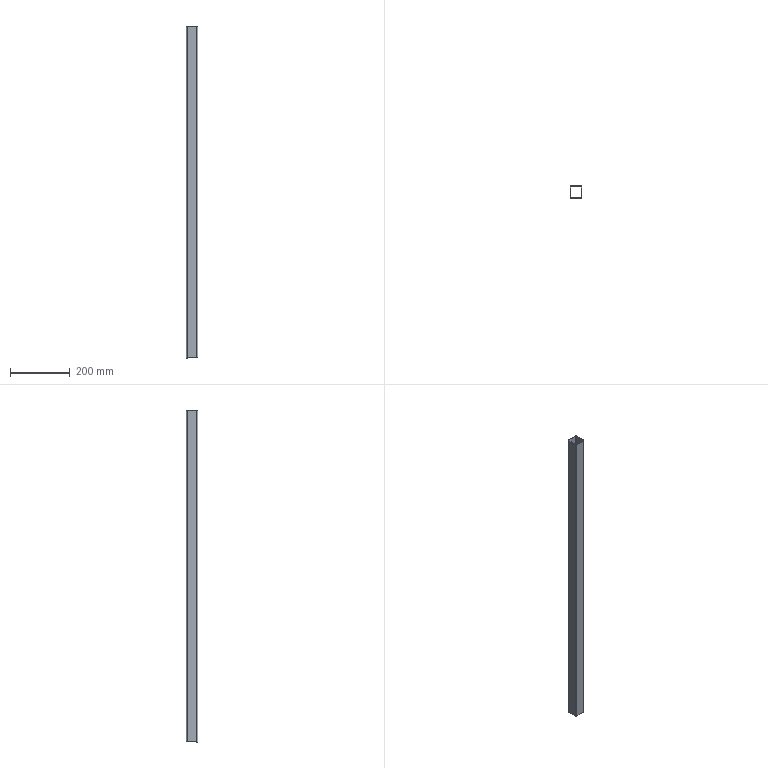Part | SolidWorks | features Fillet 2, Extrusion 1 | 1 solid | 18 faces | box 40 x 40 x 1116 mm | volume 327768 mm3 | plane 10 | cylinder 8 | commonest cylinder face diameters 4 x4 8 x4
STEP:
#1=CARTESIAN_POINT('',(20.,-16.,1116.));
#2=VERTEX_POINT('',#1);
#3=CARTESIAN_POINT('',(20.,16.,1116.));
#4=VERTEX_POINT('',#3);
#5=CARTESIAN_POINT('',(20.,20.,1116.));
#6=DIRECTION('',(0.,1.,0.));
#7=VECTOR('',#6,1000.);
#8=LINE('',#5,#7);
#9=EDGE_CURVE('',#2,#4,#8,.T.);
#10=ORIENTED_EDGE('',*,*,#9,.T.);
#11=CARTESIAN_POINT('',(16.,20.,1116.));
#12=VERTEX_POINT('',#11);
#13=CARTESIAN_POINT('',(16.,16.,1116.));
#14=DIRECTION('',(0.,0.,1.));
#15=DIRECTION('',(1.,0.,0.));
#16=AXIS2_PLACEMENT_3D('',#13,#14,#15);
#17=CIRCLE('',#16,4.);
#18=EDGE_CURVE('',#4,#12,#17,.T.);
#19=ORIENTED_EDGE('',*,*,#18,.T.);
#20=CARTESIAN_POINT('',(-16.,20.,1116.));
#21=VERTEX_POINT('',#20);
#22=CARTESIAN_POINT('',(-20.,20.,1116.));
#23=DIRECTION('',(-1.,0.,0.));
#24=VECTOR('',#23,1000.);
#25=LINE('',#22,#24);
#26=EDGE_CURVE('',#12,#21,#25,.T.);
#27=ORIENTED_EDGE('',*,*,#26,.T.);
#28=CARTESIAN_POINT('',(-20.,16.,1116.));
#29=VERTEX_POINT('',#28);
#30=CARTESIAN_POINT('',(-16.,16.,1116.));
#31=DIRECTION('',(0.,0.,1.));
#32=DIRECTION('',(1.,0.,0.));
#33=AXIS2_PLACEMENT_3D('',#30,#31,#32);
#34=CIRCLE('',#33,4.);
#35=EDGE_CURVE('',#21,#29,#34,.T.);
#36=ORIENTED_EDGE('',*,*,#35,.T.);
#37=CARTESIAN_POINT('',(-20.,-16.,1116.));
#38=VERTEX_POINT('',#37);
#39=CARTESIAN_POINT('',(-20.,20.,1116.));
#40=DIRECTION('',(0.,-1.,0.));
#41=VECTOR('',#40,1000.);
#42=LINE('',#39,#41);
#43=EDGE_CURVE('',#29,#38,#42,.T.);
#44=ORIENTED_EDGE('',*,*,#43,.T.);
#45=CARTESIAN_POINT('',(-16.,-20.,1116.));
#46=VERTEX_POINT('',#45);
#47=CARTESIAN_POINT('',(-16.,-16.,1116.));
#48=DIRECTION('',(0.,0.,1.));
#49=DIRECTION('',(1.,0.,0.));
#50=AXIS2_PLACEMENT_3D('',#47,#48,#49);
#51=CIRCLE('',#50,4.);
#52=EDGE_CURVE('',#38,#46,#51,.T.);
#53=ORIENTED_EDGE('',*,*,#52,.T.);
#54=CARTESIAN_POINT('',(16.,-20.,1116.));
#55=VERTEX_POINT('',#54);
#56=CARTESIAN_POINT('',(-20.,-20.,1116.));
#57=DIRECTION('',(1.,0.,0.));
#58=VECTOR('',#57,1000.);
#59=LINE('',#56,#58);
#60=EDGE_CURVE('',#46,#55,#59,.T.);
#61=ORIENTED_EDGE('',*,*,#60,.T.);
#62=CARTESIAN_POINT('',(16.,-16.,1116.));
#63=DIRECTION('',(0.,0.,1.));
#64=DIRECTION('',(1.,0.,0.));
#65=AXIS2_PLACEMENT_3D('',#62,#63,#64);
#66=CIRCLE('',#65,4.);
#67=EDGE_CURVE('',#55,#2,#66,.T.);
#68=ORIENTED_EDGE('',*,*,#67,.T.);
#69=EDGE_LOOP('',(#10,#19,#27,#36,#44,#53,#61,#68));
#70=FACE_OUTER_BOUND('',#69,.T.);
#71=CARTESIAN_POINT('',(16.,18.,1116.));
#72=VERTEX_POINT('',#71);
#73=CARTESIAN_POINT('',(-16.,18.,1116.));
#74=VERTEX_POINT('',#73);
#75=CARTESIAN_POINT('',(-18.,18.,1116.));
#76=DIRECTION('',(-1.,0.,0.));
#77=VECTOR('',#76,1000.);
#78=LINE('',#75,#77);
#79=EDGE_CURVE('',#72,#74,#78,.T.);
#80=ORIENTED_EDGE('',*,*,#79,.F.);
#81=CARTESIAN_POINT('',(18.,16.,1116.));
#82=VERTEX_POINT('',#81);
#83=CARTESIAN_POINT('',(16.,16.,1116.));
#84=DIRECTION('',(0.,0.,-1.));
#85=DIRECTION('',(1.,0.,0.));
#86=AXIS2_PLACEMENT_3D('',#83,#84,#85);
#87=CIRCLE('',#86,2.);
#88=EDGE_CURVE('',#72,#82,#87,.T.);
#89=ORIENTED_EDGE('',*,*,#88,.T.);
#90=CARTESIAN_POINT('',(18.,-16.,1116.));
#91=VERTEX_POINT('',#90);
#92=CARTESIAN_POINT('',(18.,18.,1116.));
#93=DIRECTION('',(0.,1.,0.));
#94=VECTOR('',#93,1000.);
#95=LINE('',#92,#94);
#96=EDGE_CURVE('',#91,#82,#95,.T.);
#97=ORIENTED_EDGE('',*,*,#96,.F.);
#98=CARTESIAN_POINT('',(16.,-18.,1116.));
#99=VERTEX_POINT('',#98);
#100=CARTESIAN_POINT('',(16.,-16.,1116.));
#101=DIRECTION('',(0.,0.,-1.));
#102=DIRECTION('',(1.,0.,0.));
#103=AXIS2_PLACEMENT_3D('',#100,#101,#102);
#104=CIRCLE('',#103,2.);
#105=EDGE_CURVE('',#91,#99,#104,.T.);
#106=ORIENTED_EDGE('',*,*,#105,.T.);
#107=CARTESIAN_POINT('',(-16.,-18.,1116.));
#108=VERTEX_POINT('',#107);
#109=CARTESIAN_POINT('',(-18.,-18.,1116.));
#110=DIRECTION('',(1.,0.,0.));
#111=VECTOR('',#110,1000.);
#112=LINE('',#109,#111);
#113=EDGE_CURVE('',#108,#99,#112,.T.);
#114=ORIENTED_EDGE('',*,*,#113,.F.);
#115=CARTESIAN_POINT('',(-18.,-16.,1116.));
#116=VERTEX_POINT('',#115);
#117=CARTESIAN_POINT('',(-16.,-16.,1116.));
#118=DIRECTION('',(0.,0.,-1.));
#119=DIRECTION('',(1.,0.,0.));
#120=AXIS2_PLACEMENT_3D('',#117,#118,#119);
#121=CIRCLE('',#120,2.);
#122=EDGE_CURVE('',#108,#116,#121,.T.);
#123=ORIENTED_EDGE('',*,*,#122,.T.);
#124=CARTESIAN_POINT('',(-18.,16.,1116.));
#125=VERTEX_POINT('',#124);
#126=CARTESIAN_POINT('',(-18.,18.,1116.));
#127=DIRECTION('',(0.,-1.,0.));
#128=VECTOR('',#127,1000.);
#129=LINE('',#126,#128);
#130=EDGE_CURVE('',#125,#116,#129,.T.);
#131=ORIENTED_EDGE('',*,*,#130,.F.);
#132=CARTESIAN_POINT('',(-16.,16.,1116.));
#133=DIRECTION('',(0.,0.,-1.));
#134=DIRECTION('',(1.,0.,0.));
#135=AXIS2_PLACEMENT_3D('',#132,#133,#134);
#136=CIRCLE('',#135,2.);
#137=EDGE_CURVE('',#125,#74,#136,.T.);
#138=ORIENTED_EDGE('',*,*,#137,.T.);
#139=EDGE_LOOP('',(#80,#89,#97,#106,#114,#123,#131,#138));
#140=FACE_BOUND('',#139,.T.);
#141=CARTESIAN_POINT('',(0.,0.,1116.));
#142=DIRECTION('',(0.,0.,1.));
#143=DIRECTION('',(1.,0.,0.));
#144=AXIS2_PLACEMENT_3D('',#141,#142,#143);
#145=PLANE('',#144);
#146=ADVANCED_FACE('',(#70,#140),#145,.T.);
#147=CARTESIAN_POINT('',(16.,20.,0.));
#148=VERTEX_POINT('',#147);
#149=CARTESIAN_POINT('',(-16.,20.,0.));
#150=VERTEX_POINT('',#149);
#151=CARTESIAN_POINT('',(-20.,20.,0.));
#152=DIRECTION('',(-1.,0.,0.));
#153=VECTOR('',#152,1000.);
#154=LINE('',#151,#153);
#155=EDGE_CURVE('',#148,#150,#154,.T.);
#156=ORIENTED_EDGE('',*,*,#155,.F.);
#157=CARTESIAN_POINT('',(20.,16.,0.));
#158=VERTEX_POINT('',#157);
#159=CARTESIAN_POINT('',(16.,16.,0.));
#160=DIRECTION('',(0.,0.,-1.));
#161=DIRECTION('',(1.,0.,0.));
#162=AXIS2_PLACEMENT_3D('',#159,#160,#161);
#163=CIRCLE('',#162,4.);
#164=EDGE_CURVE('',#148,#158,#163,.T.);
#165=ORIENTED_EDGE('',*,*,#164,.T.);
#166=CARTESIAN_POINT('',(20.,-16.,0.));
#167=VERTEX_POINT('',#166);
#168=CARTESIAN_POINT('',(20.,20.,0.));
#169=DIRECTION('',(0.,1.,0.));
#170=VECTOR('',#169,1000.);
#171=LINE('',#168,#170);
#172=EDGE_CURVE('',#167,#158,#171,.T.);
#173=ORIENTED_EDGE('',*,*,#172,.F.);
#174=CARTESIAN_POINT('',(16.,-20.,0.));
#175=VERTEX_POINT('',#174);
#176=CARTESIAN_POINT('',(16.,-16.,0.));
#177=DIRECTION('',(0.,0.,-1.));
#178=DIRECTION('',(1.,0.,0.));
#179=AXIS2_PLACEMENT_3D('',#176,#177,#178);
#180=CIRCLE('',#179,4.);
#181=EDGE_CURVE('',#167,#175,#180,.T.);
#182=ORIENTED_EDGE('',*,*,#181,.T.);
#183=CARTESIAN_POINT('',(-16.,-20.,0.));
#184=VERTEX_POINT('',#183);
#185=CARTESIAN_POINT('',(-20.,-20.,0.));
#186=DIRECTION('',(1.,0.,0.));
#187=VECTOR('',#186,1000.);
#188=LINE('',#185,#187);
#189=EDGE_CURVE('',#184,#175,#188,.T.);
#190=ORIENTED_EDGE('',*,*,#189,.F.);
#191=CARTESIAN_POINT('',(-20.,-16.,0.));
#192=VERTEX_POINT('',#191);
#193=CARTESIAN_POINT('',(-16.,-16.,0.));
#194=DIRECTION('',(0.,0.,-1.));
#195=DIRECTION('',(1.,0.,0.));
#196=AXIS2_PLACEMENT_3D('',#193,#194,#195);
#197=CIRCLE('',#196,4.);
#198=EDGE_CURVE('',#184,#192,#197,.T.);
#199=ORIENTED_EDGE('',*,*,#198,.T.);
#200=CARTESIAN_POINT('',(-20.,16.,0.));
#201=VERTEX_POINT('',#200);
#202=CARTESIAN_POINT('',(-20.,20.,0.));
#203=DIRECTION('',(0.,-1.,0.));
#204=VECTOR('',#203,1000.);
#205=LINE('',#202,#204);
#206=EDGE_CURVE('',#201,#192,#205,.T.);
#207=ORIENTED_EDGE('',*,*,#206,.F.);
#208=CARTESIAN_POINT('',(-16.,16.,0.));
#209=DIRECTION('',(0.,0.,-1.));
#210=DIRECTION('',(1.,0.,0.));
#211=AXIS2_PLACEMENT_3D('',#208,#209,#210);
#212=CIRCLE('',#211,4.);
#213=EDGE_CURVE('',#201,#150,#212,.T.);
#214=ORIENTED_EDGE('',*,*,#213,.T.);
#215=EDGE_LOOP('',(#156,#165,#173,#182,#190,#199,#207,#214));
#216=FACE_OUTER_BOUND('',#215,.T.);
#217=CARTESIAN_POINT('',(-16.,-18.,0.));
#218=VERTEX_POINT('',#217);
#219=CARTESIAN_POINT('',(16.,-18.,0.));
#220=VERTEX_POINT('',#219);
#221=CARTESIAN_POINT('',(-18.,-18.,0.));
#222=DIRECTION('',(1.,0.,0.));
#223=VECTOR('',#222,1000.);
#224=LINE('',#221,#223);
#225=EDGE_CURVE('',#218,#220,#224,.T.);
#226=ORIENTED_EDGE('',*,*,#225,.T.);
#227=CARTESIAN_POINT('',(18.,-16.,0.));
#228=VERTEX_POINT('',#227);
#229=CARTESIAN_POINT('',(16.,-16.,0.));
#230=DIRECTION('',(0.,0.,1.));
#231=DIRECTION('',(1.,0.,0.));
#232=AXIS2_PLACEMENT_3D('',#229,#230,#231);
#233=CIRCLE('',#232,2.);
#234=EDGE_CURVE('',#220,#228,#233,.T.);
#235=ORIENTED_EDGE('',*,*,#234,.T.);
#236=CARTESIAN_POINT('',(18.,16.,0.));
#237=VERTEX_POINT('',#236);
#238=CARTESIAN_POINT('',(18.,18.,0.));
#239=DIRECTION('',(0.,1.,0.));
#240=VECTOR('',#239,1000.);
#241=LINE('',#238,#240);
#242=EDGE_CURVE('',#228,#237,#241,.T.);
#243=ORIENTED_EDGE('',*,*,#242,.T.);
#244=CARTESIAN_POINT('',(16.,18.,0.));
#245=VERTEX_POINT('',#244);
#246=CARTESIAN_POINT('',(16.,16.,0.));
#247=DIRECTION('',(0.,0.,1.));
#248=DIRECTION('',(1.,0.,0.));
#249=AXIS2_PLACEMENT_3D('',#246,#247,#248);
#250=CIRCLE('',#249,2.);
#251=EDGE_CURVE('',#237,#245,#250,.T.);
#252=ORIENTED_EDGE('',*,*,#251,.T.);
#253=CARTESIAN_POINT('',(-16.,18.,0.));
#254=VERTEX_POINT('',#253);
#255=CARTESIAN_POINT('',(-18.,18.,0.));
#256=DIRECTION('',(-1.,0.,0.));
#257=VECTOR('',#256,1000.);
#258=LINE('',#255,#257);
#259=EDGE_CURVE('',#245,#254,#258,.T.);
#260=ORIENTED_EDGE('',*,*,#259,.T.);
#261=CARTESIAN_POINT('',(-18.,16.,0.));
#262=VERTEX_POINT('',#261);
#263=CARTESIAN_POINT('',(-16.,16.,0.));
#264=DIRECTION('',(0.,0.,1.));
#265=DIRECTION('',(1.,0.,0.));
#266=AXIS2_PLACEMENT_3D('',#263,#264,#265);
#267=CIRCLE('',#266,2.);
#268=EDGE_CURVE('',#254,#262,#267,.T.);
#269=ORIENTED_EDGE('',*,*,#268,.T.);
#270=CARTESIAN_POINT('',(-18.,-16.,0.));
#271=VERTEX_POINT('',#270);
#272=CARTESIAN_POINT('',(-18.,18.,0.));
#273=DIRECTION('',(0.,-1.,0.));
#274=VECTOR('',#273,1000.);
#275=LINE('',#272,#274);
#276=EDGE_CURVE('',#262,#271,#275,.T.);
#277=ORIENTED_EDGE('',*,*,#276,.T.);
#278=CARTESIAN_POINT('',(-16.,-16.,0.));
#279=DIRECTION('',(0.,0.,1.));
#280=DIRECTION('',(1.,0.,0.));
#281=AXIS2_PLACEMENT_3D('',#278,#279,#280);
#282=CIRCLE('',#281,2.);
#283=EDGE_CURVE('',#271,#218,#282,.T.);
#284=ORIENTED_EDGE('',*,*,#283,.T.);
#285=EDGE_LOOP('',(#226,#235,#243,#252,#260,#269,#277,#284));
#286=FACE_BOUND('',#285,.T.);
#287=CARTESIAN_POINT('',(0.,0.,0.));
#288=DIRECTION('',(0.,0.,1.));
#289=DIRECTION('',(1.,0.,0.));
#290=AXIS2_PLACEMENT_3D('',#287,#288,#289);
#291=PLANE('',#290);
#292=ADVANCED_FACE('',(#216,#286),#291,.F.);
#293=ORIENTED_EDGE('',*,*,#172,.T.);
#294=CARTESIAN_POINT('',(20.,16.,1116.));
#295=DIRECTION('',(0.,0.,1.));
#296=VECTOR('',#295,1000.);
#297=LINE('',#294,#296);
#298=EDGE_CURVE('',#158,#4,#297,.T.);
#299=ORIENTED_EDGE('',*,*,#298,.T.);
#300=ORIENTED_EDGE('',*,*,#9,.F.);
#301=CARTESIAN_POINT('',(20.,-16.,1116.));
#302=DIRECTION('',(0.,0.,-1.));
#303=VECTOR('',#302,1000.);
#304=LINE('',#301,#303);
#305=EDGE_CURVE('',#2,#167,#304,.T.);
#306=ORIENTED_EDGE('',*,*,#305,.T.);
#307=EDGE_LOOP('',(#293,#299,#300,#306));
#308=FACE_OUTER_BOUND('',#307,.T.);
#309=CARTESIAN_POINT('',(20.,20.,1116.));
#310=DIRECTION('',(-1.,0.,0.));
#311=DIRECTION('',(0.,0.,1.));
#312=AXIS2_PLACEMENT_3D('',#309,#310,#311);
#313=PLANE('',#312);
#314=ADVANCED_FACE('',(#308),#313,.F.);
#315=ORIENTED_EDGE('',*,*,#26,.F.);
#316=CARTESIAN_POINT('',(16.,20.,1116.));
#317=DIRECTION('',(0.,0.,-1.));
#318=VECTOR('',#317,1000.);
#319=LINE('',#316,#318);
#320=EDGE_CURVE('',#12,#148,#319,.T.);
#321=ORIENTED_EDGE('',*,*,#320,.T.);
#322=ORIENTED_EDGE('',*,*,#155,.T.);
#323=CARTESIAN_POINT('',(-16.,20.,1116.));
#324=DIRECTION('',(0.,0.,1.));
#325=VECTOR('',#324,1000.);
#326=LINE('',#323,#325);
#327=EDGE_CURVE('',#150,#21,#326,.T.);
#328=ORIENTED_EDGE('',*,*,#327,.T.);
#329=EDGE_LOOP('',(#315,#321,#322,#328));
#330=FACE_OUTER_BOUND('',#329,.T.);
#331=CARTESIAN_POINT('',(-20.,20.,1116.));
#332=DIRECTION('',(0.,-1.,0.));
#333=DIRECTION('',(0.,0.,-1.));
#334=AXIS2_PLACEMENT_3D('',#331,#332,#333);
#335=PLANE('',#334);
#336=ADVANCED_FACE('',(#330),#335,.F.);
#337=ORIENTED_EDGE('',*,*,#43,.F.);
#338=CARTESIAN_POINT('',(-20.,16.,1116.));
#339=DIRECTION('',(0.,0.,-1.));
#340=VECTOR('',#339,1000.);
#341=LINE('',#338,#340);
#342=EDGE_CURVE('',#29,#201,#341,.T.);
#343=ORIENTED_EDGE('',*,*,#342,.T.);
#344=ORIENTED_EDGE('',*,*,#206,.T.);
#345=CARTESIAN_POINT('',(-20.,-16.,1116.));
#346=DIRECTION('',(0.,0.,1.));
#347=VECTOR('',#346,1000.);
#348=LINE('',#345,#347);
#349=EDGE_CURVE('',#192,#38,#348,.T.);
#350=ORIENTED_EDGE('',*,*,#349,.T.);
#351=EDGE_LOOP('',(#337,#343,#344,#350));
#352=FACE_OUTER_BOUND('',#351,.T.);
#353=CARTESIAN_POINT('',(-20.,20.,1116.));
#354=DIRECTION('',(1.,0.,0.));
#355=DIRECTION('',(0.,0.,-1.));
#356=AXIS2_PLACEMENT_3D('',#353,#354,#355);
#357=PLANE('',#356);
#358=ADVANCED_FACE('',(#352),#357,.F.);
#359=ORIENTED_EDGE('',*,*,#189,.T.);
#360=CARTESIAN_POINT('',(16.,-20.,1116.));
#361=DIRECTION('',(0.,0.,1.));
#362=VECTOR('',#361,1000.);
#363=LINE('',#360,#362);
#364=EDGE_CURVE('',#175,#55,#363,.T.);
#365=ORIENTED_EDGE('',*,*,#364,.T.);
#366=ORIENTED_EDGE('',*,*,#60,.F.);
#367=CARTESIAN_POINT('',(-16.,-20.,1116.));
#368=DIRECTION('',(0.,0.,-1.));
#369=VECTOR('',#368,1000.);
#370=LINE('',#367,#369);
#371=EDGE_CURVE('',#46,#184,#370,.T.);
#372=ORIENTED_EDGE('',*,*,#371,.T.);
#373=EDGE_LOOP('',(#359,#365,#366,#372));
#374=FACE_OUTER_BOUND('',#373,.T.);
#375=CARTESIAN_POINT('',(-20.,-20.,1116.));
#376=DIRECTION('',(0.,1.,0.));
#377=DIRECTION('',(0.,0.,1.));
#378=AXIS2_PLACEMENT_3D('',#375,#376,#377);
#379=PLANE('',#378);
#380=ADVANCED_FACE('',(#374),#379,.F.);
#381=ORIENTED_EDGE('',*,*,#96,.T.);
#382=CARTESIAN_POINT('',(18.,16.,0.));
#383=DIRECTION('',(0.,0.,-1.));
#384=VECTOR('',#383,1000.);
#385=LINE('',#382,#384);
#386=EDGE_CURVE('',#82,#237,#385,.T.);
#387=ORIENTED_EDGE('',*,*,#386,.T.);
#388=ORIENTED_EDGE('',*,*,#242,.F.);
#389=CARTESIAN_POINT('',(18.,-16.,1116.));
#390=DIRECTION('',(0.,0.,1.));
#391=VECTOR('',#390,1000.);
#392=LINE('',#389,#391);
#393=EDGE_CURVE('',#228,#91,#392,.T.);
#394=ORIENTED_EDGE('',*,*,#393,.T.);
#395=EDGE_LOOP('',(#381,#387,#388,#394));
#396=FACE_OUTER_BOUND('',#395,.T.);
#397=CARTESIAN_POINT('',(18.,18.,1116.));
#398=DIRECTION('',(-1.,0.,0.));
#399=DIRECTION('',(0.,0.,1.));
#400=AXIS2_PLACEMENT_3D('',#397,#398,#399);
#401=PLANE('',#400);
#402=ADVANCED_FACE('',(#396),#401,.T.);
#403=ORIENTED_EDGE('',*,*,#259,.F.);
#404=CARTESIAN_POINT('',(16.,18.,1116.));
#405=DIRECTION('',(0.,0.,1.));
#406=VECTOR('',#405,1000.);
#407=LINE('',#404,#406);
#408=EDGE_CURVE('',#245,#72,#407,.T.);
#409=ORIENTED_EDGE('',*,*,#408,.T.);
#410=ORIENTED_EDGE('',*,*,#79,.T.);
#411=CARTESIAN_POINT('',(-16.,18.,0.));
#412=DIRECTION('',(0.,0.,-1.));
#413=VECTOR('',#412,1000.);
#414=LINE('',#411,#413);
#415=EDGE_CURVE('',#74,#254,#414,.T.);
#416=ORIENTED_EDGE('',*,*,#415,.T.);
#417=EDGE_LOOP('',(#403,#409,#410,#416));
#418=FACE_OUTER_BOUND('',#417,.T.);
#419=CARTESIAN_POINT('',(-18.,18.,1116.));
#420=DIRECTION('',(0.,-1.,0.));
#421=DIRECTION('',(0.,0.,-1.));
#422=AXIS2_PLACEMENT_3D('',#419,#420,#421);
#423=PLANE('',#422);
#424=ADVANCED_FACE('',(#418),#423,.T.);
#425=ORIENTED_EDGE('',*,*,#276,.F.);
#426=CARTESIAN_POINT('',(-18.,16.,1116.));
#427=DIRECTION('',(0.,0.,1.));
#428=VECTOR('',#427,1000.);
#429=LINE('',#426,#428);
#430=EDGE_CURVE('',#262,#125,#429,.T.);
#431=ORIENTED_EDGE('',*,*,#430,.T.);
#432=ORIENTED_EDGE('',*,*,#130,.T.);
#433=CARTESIAN_POINT('',(-18.,-16.,0.));
#434=DIRECTION('',(0.,0.,-1.));
#435=VECTOR('',#434,1000.);
#436=LINE('',#433,#435);
#437=EDGE_CURVE('',#116,#271,#436,.T.);
#438=ORIENTED_EDGE('',*,*,#437,.T.);
#439=EDGE_LOOP('',(#425,#431,#432,#438));
#440=FACE_OUTER_BOUND('',#439,.T.);
#441=CARTESIAN_POINT('',(-18.,18.,1116.));
#442=DIRECTION('',(1.,0.,0.));
#443=DIRECTION('',(0.,0.,-1.));
#444=AXIS2_PLACEMENT_3D('',#441,#442,#443);
#445=PLANE('',#444);
#446=ADVANCED_FACE('',(#440),#445,.T.);
#447=ORIENTED_EDGE('',*,*,#225,.F.);
#448=CARTESIAN_POINT('',(-16.,-18.,1116.));
#449=DIRECTION('',(0.,0.,1.));
#450=VECTOR('',#449,1000.);
#451=LINE('',#448,#450);
#452=EDGE_CURVE('',#218,#108,#451,.T.);
#453=ORIENTED_EDGE('',*,*,#452,.T.);
#454=ORIENTED_EDGE('',*,*,#113,.T.);
#455=CARTESIAN_POINT('',(16.,-18.,0.));
#456=DIRECTION('',(0.,0.,-1.));
#457=VECTOR('',#456,1000.);
#458=LINE('',#455,#457);
#459=EDGE_CURVE('',#99,#220,#458,.T.);
#460=ORIENTED_EDGE('',*,*,#459,.T.);
#461=EDGE_LOOP('',(#447,#453,#454,#460));
#462=FACE_OUTER_BOUND('',#461,.T.);
#463=CARTESIAN_POINT('',(-18.,-18.,1116.));
#464=DIRECTION('',(0.,1.,0.));
#465=DIRECTION('',(0.,0.,1.));
#466=AXIS2_PLACEMENT_3D('',#463,#464,#465);
#467=PLANE('',#466);
#468=ADVANCED_FACE('',(#462),#467,.T.);
#469=ORIENTED_EDGE('',*,*,#88,.F.);
#470=ORIENTED_EDGE('',*,*,#408,.F.);
#471=ORIENTED_EDGE('',*,*,#251,.F.);
#472=ORIENTED_EDGE('',*,*,#386,.F.);
#473=EDGE_LOOP('',(#469,#470,#471,#472));
#474=FACE_OUTER_BOUND('',#473,.T.);
#475=CARTESIAN_POINT('',(16.,16.,1116.));
#476=DIRECTION('',(0.,0.,1.));
#477=DIRECTION('',(1.,0.,0.));
#478=AXIS2_PLACEMENT_3D('',#475,#476,#477);
#479=CYLINDRICAL_SURFACE('',#478,2.);
#480=ADVANCED_FACE('',(#474),#479,.F.);
#481=ORIENTED_EDGE('',*,*,#137,.F.);
#482=ORIENTED_EDGE('',*,*,#430,.F.);
#483=ORIENTED_EDGE('',*,*,#268,.F.);
#484=ORIENTED_EDGE('',*,*,#415,.F.);
#485=EDGE_LOOP('',(#481,#482,#483,#484));
#486=FACE_OUTER_BOUND('',#485,.T.);
#487=CARTESIAN_POINT('',(-16.,16.,1116.));
#488=DIRECTION('',(0.,0.,1.));
#489=DIRECTION('',(1.,0.,0.));
#490=AXIS2_PLACEMENT_3D('',#487,#488,#489);
#491=CYLINDRICAL_SURFACE('',#490,2.);
#492=ADVANCED_FACE('',(#486),#491,.F.);
#493=ORIENTED_EDGE('',*,*,#122,.F.);
#494=ORIENTED_EDGE('',*,*,#452,.F.);
#495=ORIENTED_EDGE('',*,*,#283,.F.);
#496=ORIENTED_EDGE('',*,*,#437,.F.);
#497=EDGE_LOOP('',(#493,#494,#495,#496));
#498=FACE_OUTER_BOUND('',#497,.T.);
#499=CARTESIAN_POINT('',(-16.,-16.,1116.));
#500=DIRECTION('',(0.,0.,1.));
#501=DIRECTION('',(1.,0.,0.));
#502=AXIS2_PLACEMENT_3D('',#499,#500,#501);
#503=CYLINDRICAL_SURFACE('',#502,2.);
#504=ADVANCED_FACE('',(#498),#503,.F.);
#505=ORIENTED_EDGE('',*,*,#105,.F.);
#506=ORIENTED_EDGE('',*,*,#393,.F.);
#507=ORIENTED_EDGE('',*,*,#234,.F.);
#508=ORIENTED_EDGE('',*,*,#459,.F.);
#509=EDGE_LOOP('',(#505,#506,#507,#508));
#510=FACE_OUTER_BOUND('',#509,.T.);
#511=CARTESIAN_POINT('',(16.,-16.,1116.));
#512=DIRECTION('',(0.,0.,1.));
#513=DIRECTION('',(1.,0.,0.));
#514=AXIS2_PLACEMENT_3D('',#511,#512,#513);
#515=CYLINDRICAL_SURFACE('',#514,2.);
#516=ADVANCED_FACE('',(#510),#515,.F.);
#517=ORIENTED_EDGE('',*,*,#18,.F.);
#518=ORIENTED_EDGE('',*,*,#298,.F.);
#519=ORIENTED_EDGE('',*,*,#164,.F.);
#520=ORIENTED_EDGE('',*,*,#320,.F.);
#521=EDGE_LOOP('',(#517,#518,#519,#520));
#522=FACE_OUTER_BOUND('',#521,.T.);
#523=CARTESIAN_POINT('',(16.,16.,1116.));
#524=DIRECTION('',(0.,0.,-1.));
#525=DIRECTION('',(-1.,0.,0.));
#526=AXIS2_PLACEMENT_3D('',#523,#524,#525);
#527=CYLINDRICAL_SURFACE('',#526,4.);
#528=ADVANCED_FACE('',(#522),#527,.T.);
#529=ORIENTED_EDGE('',*,*,#67,.F.);
#530=ORIENTED_EDGE('',*,*,#364,.F.);
#531=ORIENTED_EDGE('',*,*,#181,.F.);
#532=ORIENTED_EDGE('',*,*,#305,.F.);
#533=EDGE_LOOP('',(#529,#530,#531,#532));
#534=FACE_OUTER_BOUND('',#533,.T.);
#535=CARTESIAN_POINT('',(16.,-16.,1116.));
#536=DIRECTION('',(0.,0.,-1.));
#537=DIRECTION('',(-1.,0.,0.));
#538=AXIS2_PLACEMENT_3D('',#535,#536,#537);
#539=CYLINDRICAL_SURFACE('',#538,4.);
#540=ADVANCED_FACE('',(#534),#539,.T.);
#541=ORIENTED_EDGE('',*,*,#35,.F.);
#542=ORIENTED_EDGE('',*,*,#327,.F.);
#543=ORIENTED_EDGE('',*,*,#213,.F.);
#544=ORIENTED_EDGE('',*,*,#342,.F.);
#545=EDGE_LOOP('',(#541,#542,#543,#544));
#546=FACE_OUTER_BOUND('',#545,.T.);
#547=CARTESIAN_POINT('',(-16.,16.,1116.));
#548=DIRECTION('',(0.,0.,-1.));
#549=DIRECTION('',(-1.,0.,0.));
#550=AXIS2_PLACEMENT_3D('',#547,#548,#549);
#551=CYLINDRICAL_SURFACE('',#550,4.);
#552=ADVANCED_FACE('',(#546),#551,.T.);
#553=ORIENTED_EDGE('',*,*,#52,.F.);
#554=ORIENTED_EDGE('',*,*,#349,.F.);
#555=ORIENTED_EDGE('',*,*,#198,.F.);
#556=ORIENTED_EDGE('',*,*,#371,.F.);
#557=EDGE_LOOP('',(#553,#554,#555,#556));
#558=FACE_OUTER_BOUND('',#557,.T.);
#559=CARTESIAN_POINT('',(-16.,-16.,1116.));
#560=DIRECTION('',(0.,0.,-1.));
#561=DIRECTION('',(-1.,0.,0.));
#562=AXIS2_PLACEMENT_3D('',#559,#560,#561);
#563=CYLINDRICAL_SURFACE('',#562,4.);
#564=ADVANCED_FACE('',(#558),#563,.T.);
#565=CLOSED_SHELL('',(#146,#292,#314,#336,#358,#380,#402,#424,#446,#468,#480,#492,#504,#516,#528,#540,#552,#564));
#566=MANIFOLD_SOLID_BREP('',#565);
#567=CARTESIAN_POINT('',(0.,0.,0.));
#568=DIRECTION('',(0.,0.,1.));
#569=DIRECTION('',(1.,0.,0.));
#570=AXIS2_PLACEMENT_3D('',#567,#568,#569);
#571=(LENGTH_UNIT()NAMED_UNIT(*)SI_UNIT(.MILLI.,.METRE.));
#572=UNCERTAINTY_MEASURE_WITH_UNIT(LENGTH_MEASURE(0.00001),#571,'','');
#573=(NAMED_UNIT(*)PLANE_ANGLE_UNIT()SI_UNIT($,.RADIAN.));
#574=(NAMED_UNIT(*)SI_UNIT($,.STERADIAN.)SOLID_ANGLE_UNIT());
#575=(GEOMETRIC_REPRESENTATION_CONTEXT(3)GLOBAL_UNCERTAINTY_ASSIGNED_CONTEXT((#572))GLOBAL_UNIT_ASSIGNED_CONTEXT((#571,#573,#574))REPRESENTATION_CONTEXT('',''));
#576=ADVANCED_BREP_SHAPE_REPRESENTATION('',(#566,#570),#575);